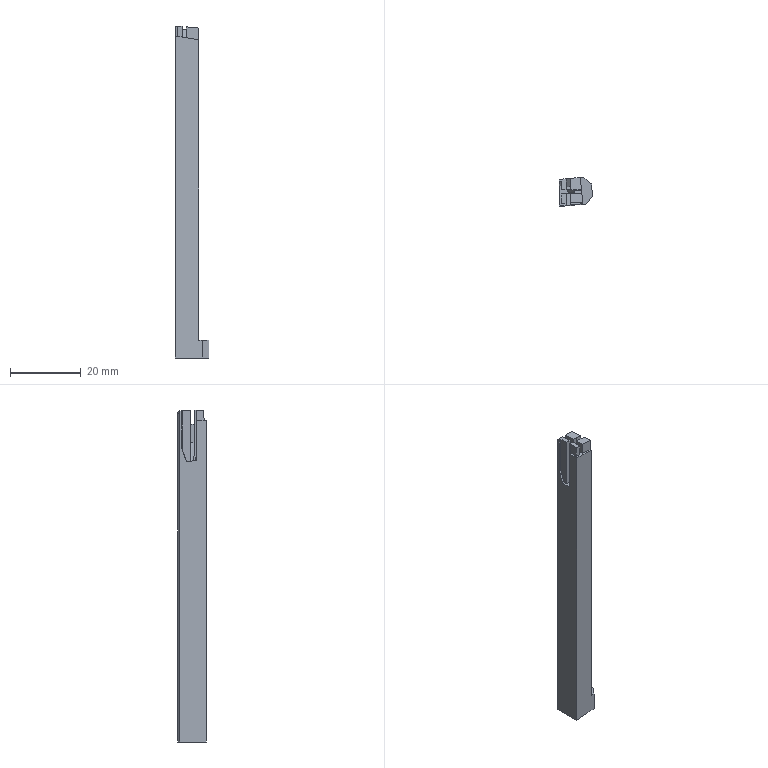Part | STEP file | P011002M010-000 | 1 solid | 41 faces | box 9.465 x 8.201 x 94.193 mm | volume 4408 mm3 | spline 30 | plane 11